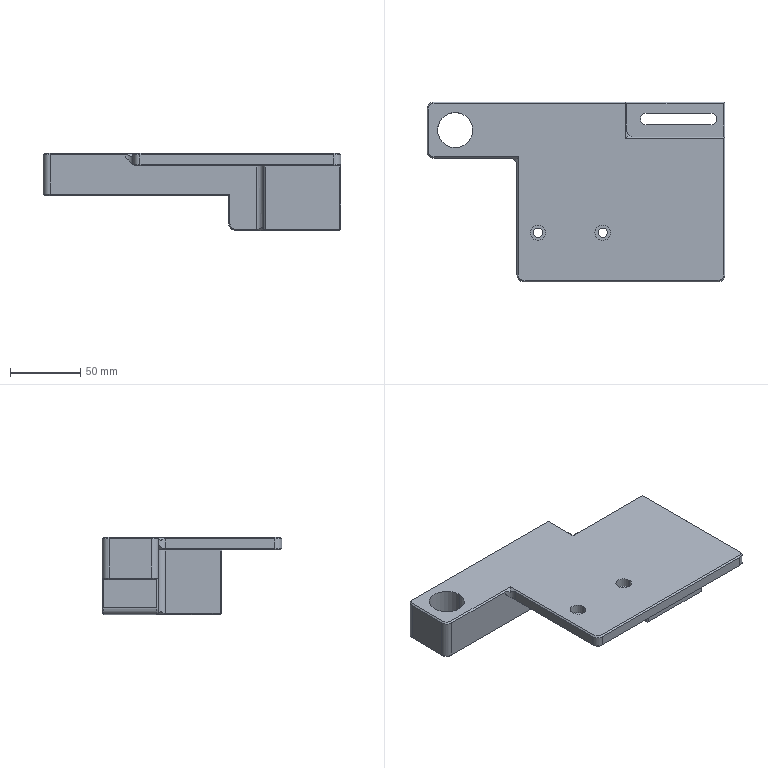NC program | NX | posted with a generic post | part box 212 x 128 x 55 mm
Lines 40 to 1041 of 7327:
(ZLEVEL_PROFILE , TOOL : D17R0.8)
N66 T19 M6
N68 G54
N70 G17 G0 G90 X-34.204 Y-75.847 S2000 M3
N72 G43 Z30. H19
N74 Z-0.299
N76 G94 G1 X-35.548 Y-73.385 F1000.
N78 G3 X-37. Y-72.5 R1.7
N80 G1 X-37.377 Y-72.491 F2000.
N82 X-39.204 Y-72.315
N84 G2 X-41.763 Y-71.628 R16.725
N86 X-44.137 Y-70.455 R17.555
N88 X-46.243 Y-68.833 R16.661
N90 X-48.008 Y-66.81 R16.904
N92 X-49.323 Y-64.502 R16.126
N94 X-50.15 Y-62.04 R17.33
N96 X-50.5 Y-59.144 R17.117
N98 G1 Y15.5
N100 X-100.985
N102 X-101.383 Y15.509
N104 X-103.25 Y15.692
N106 G2 X-105.769 Y16.375 R18.316
N108 X-110.251 Y19.173 R14.115
N110 X-111.999 Y21.178 R16.782
N112 X-113.297 Y23.438 R17.54
N114 X-114.152 Y25.971 R16.756
N116 X-114.49 Y28.605 R16.66
N118 G1 X-114.5 Y29.
N120 X-114.496 Y29.035
N122 X-114.498 Y30.056
N124 X-114.499 Y30.558
N126 G3 X-115.354 Y32.027 R1.7
N128 G1 X-117.608 Y33.32
N130 G0 X-117.607 Y33.322 Z-0.598
N132 G1 X-115.353 Y32.028 F1000.
N134 G2 X-114.499 Y30.558 R1.7
N136 G1 X-114.498 Y30.056 F2000.
N138 X-114.497 Y29.035
N140 X-114.5 Y29.
N142 X-114.49 Y28.605
N144 G3 X-114.152 Y25.971 R16.408
N146 X-113.297 Y23.438 R15.504
N148 X-111.999 Y21.178 R17.275
N150 X-110.251 Y19.173 R16.617
N152 X-105.769 Y16.375 R14.059
N154 X-103.25 Y15.692 R17.985
N156 G1 X-101.383 Y15.509
N158 X-100.985 Y15.5
N160 X-50.5
N162 Y-59.138
N164 G3 X-50.15 Y-62.04 R16.924
N166 G1 X-50.061 Y-62.353
N168 X-49.627 Y-63.765
N170 X-49.592 Y-63.858
N172 G3 X-48.318 Y-66.377 R16.221
N174 X-46.243 Y-68.833 R16.659
N176 X-44.137 Y-70.455 R16.48
N178 X-41.763 Y-71.628 R17.111
N180 X-39.204 Y-72.315 R16.672
N182 G1 X-37.377 Y-72.491
N184 X-37. Y-72.5
N186 G2 X-35.548 Y-73.385 R1.7
N188 G1 X-34.208 Y-75.839
N190 G0 X-34.207 Y-75.843 Z-0.897
N192 G1 X-35.548 Y-73.385 F1000.
N194 G3 X-37. Y-72.5 R1.7
N196 G1 X-37.377 Y-72.491 F2000.
N198 X-39.204 Y-72.315
N200 G2 X-41.763 Y-71.628 R16.772
N202 X-44.137 Y-70.455 R16.925
N204 X-46.243 Y-68.833 R16.304
N206 X-48.008 Y-66.81 R16.476
N208 X-50.134 Y-62.108 R13.885
N210 X-50.5 Y-59.121 R16.437
N212 G1 Y15.5
N214 X-100.985
N216 X-101.383 Y15.509
N218 X-103.25 Y15.692
N220 G2 X-105.769 Y16.375 R17.578
N222 X-110.251 Y19.173 R14.002
N224 X-111.999 Y21.178 R16.455
N226 X-113.297 Y23.438 R17.026
N228 X-114.152 Y25.971 R15.355
N230 X-114.49 Y28.605 R17.016
N232 G1 X-114.5 Y29.
N234 X-114.498 Y30.056
N236 X-114.499 Y30.558
N238 G3 X-115.352 Y32.028 R1.7
N240 G1 X-117.607 Y33.325
N242 G0 X-117.634 Y33.343 Z-1.196
N244 G1 X-115.351 Y32.029 F1000.
N246 G2 X-114.499 Y30.558 R1.7
N248 G1 Y30.056 F2000.
N250 X-114.5 Y29.
N252 X-114.49 Y28.605
N254 G3 X-114.152 Y25.971 R16.763
N256 X-112.816 Y22.397 R16.562
N258 X-110.251 Y19.173 R16.296
N260 X-105.769 Y16.375 R13.947
N262 X-103.218 Y15.687 R17.241
N264 G1 X-101.383 Y15.509
N266 X-100.985 Y15.5
N268 X-50.5
N270 Y-59.119
N272 G3 X-50.15 Y-62.04 R16.449
N274 X-49.323 Y-64.503 R16.842
N276 X-47.755 Y-67.18 R16.253
N278 X-44.137 Y-70.455 R14.338
N280 X-41.763 Y-71.628 R16.744
N282 X-39.204 Y-72.315 R16.566
N284 G1 X-37.377 Y-72.491
N286 X-37. Y-72.5
N288 G2 X-35.548 Y-73.385 R1.7
N290 G1 X-34.206 Y-75.844
N292 G0 X-34.205 Y-75.846 Z-1.495
N294 G1 X-35.548 Y-73.385 F1000.
N296 G3 X-37. Y-72.5 R1.7
N298 G1 X-37.377 Y-72.491 F2000.
N300 X-39.204 Y-72.315
N302 G2 X-41.763 Y-71.628 R16.392
N304 X-44.137 Y-70.455 R16.512
N306 X-47.853 Y-67.036 R14.045
N308 X-49.323 Y-64.503 R15.704
N310 X-50.15 Y-62.04 R16.586
N312 X-50.5 Y-59.105 R16.167
N314 G1 Y15.5
N316 X-100.985
N318 X-101.431 Y15.51
N320 X-103.25 Y15.692
N322 G2 X-105.769 Y16.375 R16.963
N324 X-110.251 Y19.173 R13.91
N326 X-112.823 Y22.412 R16.137
N328 X-114.152 Y25.971 R16.822
N330 X-114.49 Y28.605 R16.493
N332 G1 X-114.5 Y29.
N334 X-114.499 Y30.056
N336 Y30.558
N338 G3 X-115.35 Y32.029 R1.7
N340 G1 X-117.839 Y33.464
N342 G0 X-117.899 Y33.502 Z-1.793
N344 G1 X-115.349 Y32.03 F1000.
N346 G2 X-114.499 Y30.558 R1.7
N348 G1 Y30.056 F2000.
N350 X-114.5 Y29.
N352 G3 X-100.985 Y15.5 R13.507
N354 G1 X-50.5
N356 Y-59.882
N358 X-50.31 Y-61.241
N360 X-50.268 Y-61.476
N362 G3 X-37. Y-72.5 R13.504
N364 G2 X-35.528 Y-73.351 R1.7
N366 G1 X-34.058 Y-75.9
N368 G0 X-34.056 Z-2.092
N370 G1 X-35.528 Y-73.35 F1000.
N372 G3 X-37. Y-72.5 R1.7
N374 G2 X-50.5 Y-59. R13.5 F2000.
N376 G1 Y15.5
N378 X-101.
N380 G2 X-114.5 Y29. R13.5
N382 G1 Y29.553
N384 X-114.499 Y30.558
N386 G3 X-115.348 Y32.031 R1.7
N388 G1 X-117.9 Y33.507
N390 G0 Z-2.391
N392 G1 X-115.348 Y32.031 F1000.
N394 G2 X-114.499 Y30.558 R1.7
N396 G1 X-114.5 Y29.553 F2000.
N398 Y29.
N400 G3 X-101. Y15.5 R13.5
N402 G1 X-50.5
N404 Y-59.
N406 G3 X-37. Y-72.5 R13.5
N408 G2 X-35.528 Y-73.35 R1.7
N410 G1 X-34.056 Y-75.9
N412 G0 Z-2.69
N414 G1 X-35.528 Y-73.35 F1000.
N416 G3 X-37. Y-72.5 R1.7
N418 G2 X-50.5 Y-59. R13.5 F2000.
N420 G1 Y15.5
N422 X-101.
N424 G2 X-114.5 Y29. R13.5
N426 G1 Y29.553
N428 X-114.499 Y30.558
N430 G3 X-115.348 Y32.031 R1.7
N432 G1 X-117.9 Y33.507
N434 G0 Z-2.989
N436 G1 X-115.348 Y32.031 F1000.
N438 G2 X-114.499 Y30.558 R1.7
N440 G1 X-114.5 Y29.553 F2000.
N442 Y29.
N444 G3 X-101. Y15.5 R13.5
N446 G1 X-50.5
N448 Y-59.
N450 G3 X-37. Y-72.5 R13.5
N452 G2 X-35.528 Y-73.35 R1.7
N454 G1 X-34.056 Y-75.9
N456 G0 Z-3.288
N458 G1 X-35.528 Y-73.35 F1000.
N460 G3 X-37. Y-72.5 R1.7
N462 G2 X-50.5 Y-59. R13.5 F2000.
N464 G1 Y15.5
N466 X-101.
N468 G2 X-114.5 Y29. R13.5
N470 G1 Y29.553
N472 X-114.499 Y30.558
N474 G3 X-115.348 Y32.031 R1.7
N476 G1 X-117.9 Y33.507
N478 G0 Z-3.587
N480 G1 X-115.348 Y32.031 F1000.
N482 G2 X-114.499 Y30.558 R1.7
N484 G1 X-114.5 Y29.553 F2000.
N486 Y29.
N488 G3 X-101. Y15.5 R13.5
N490 G1 X-50.5
N492 Y-59.
N494 G3 X-37. Y-72.5 R13.5
N496 G2 X-35.528 Y-73.35 R1.7
N498 G1 X-34.056 Y-75.9
N500 G0 Z-3.886
N502 G1 X-35.528 Y-73.35 F1000.
N504 G3 X-37. Y-72.5 R1.7
N506 G2 X-50.5 Y-59. R13.5 F2000.
N508 G1 Y15.5
N510 X-101.
N512 G2 X-114.5 Y29. R13.5
N514 G1 Y29.553
N516 X-114.499 Y30.558
N518 G3 X-115.348 Y32.031 R1.7
N520 G1 X-117.9 Y33.507
N522 G0 Z-4.185
N524 G1 X-115.348 Y32.031 F1000.
N526 G2 X-114.499 Y30.558 R1.7
N528 G1 X-114.5 Y29.553 F2000.
N530 Y29.
N532 G3 X-101. Y15.5 R13.5
N534 G1 X-50.5
N536 Y-59.
N538 G3 X-37. Y-72.5 R13.5
N540 G2 X-35.528 Y-73.35 R1.7
N542 G1 X-34.056 Y-75.9
N544 G0 Z-4.484
N546 G1 X-35.528 Y-73.35 F1000.
N548 G3 X-37. Y-72.5 R1.7
N550 G2 X-50.5 Y-59. R13.5 F2000.
N552 G1 Y15.5
N554 X-101.
N556 G2 X-114.5 Y29. R13.5
N558 G1 Y29.553
N560 X-114.499 Y30.558
N562 G3 X-115.348 Y32.031 R1.7
N564 G1 X-117.9 Y33.507
N566 G0 Z-4.783
N568 G1 X-115.348 Y32.031 F1000.
N570 G2 X-114.499 Y30.558 R1.7
N572 G1 X-114.5 Y29.553 F2000.
N574 Y29.
N576 G3 X-101. Y15.5 R13.5
N578 G1 X-50.5
N580 Y-59.
N582 G3 X-37. Y-72.5 R13.5
N584 G2 X-35.528 Y-73.35 R1.7
N586 G1 X-34.056 Y-75.9
N588 G0 Z-5.082
N590 G1 X-35.528 Y-73.35 F1000.
N592 G3 X-37. Y-72.5 R1.7
N594 G2 X-50.5 Y-59. R13.5 F2000.
N596 G1 Y15.5
N598 X-101.
N600 G2 X-114.5 Y29. R13.5
N602 G1 Y29.553
N604 X-114.499 Y30.558
N606 G3 X-115.348 Y32.031 R1.7
N608 G1 X-117.9 Y33.507
N610 G0 Z-5.38
N612 G1 X-115.348 Y32.031 F1000.
N614 G2 X-114.499 Y30.558 R1.7
N616 G1 X-114.5 Y29.553 F2000.
N618 Y29.
N620 G3 X-101. Y15.5 R13.5
N622 G1 X-50.5
N624 Y-59.
N626 G3 X-37. Y-72.5 R13.5
N628 G2 X-35.528 Y-73.35 R1.7
N630 G1 X-34.056 Y-75.9
N632 G0 Z-5.679
N634 G1 X-35.528 Y-73.35 F1000.
N636 G3 X-37. Y-72.5 R1.7
N638 G2 X-50.5 Y-59. R13.5 F2000.
N640 G1 Y15.5
N642 X-101.
N644 G2 X-114.5 Y29. R13.5
N646 G1 Y29.553
N648 X-114.499 Y30.558
N650 G3 X-115.348 Y32.031 R1.7
N652 G1 X-117.9 Y33.507
N654 G0 Y33.506 Z-5.978
N656 G1 X-115.348 Y32.031 F1000.
N658 G2 X-114.499 Y30.558 R1.7
N660 G1 X-114.5 Y29.553 F2000.
N662 Y29.
N664 G3 X-101. Y15.5 R13.5
N666 G1 X-50.5
N668 Y-59.
N670 G3 X-37. Y-72.5 R13.5
N672 G2 X-35.528 Y-73.35 R1.7
N674 G1 X-34.056 Y-75.9
N676 G0 Z-6.277
N678 G1 X-35.528 Y-73.35 F1000.
N680 G3 X-37. Y-72.5 R1.7
N682 G2 X-50.5 Y-59. R13.5 F2000.
N684 G1 Y15.5
N686 X-101.
N688 G2 X-114.5 Y29. R13.5
N690 G1 Y29.553
N692 X-114.499 Y30.558
N694 G3 X-115.348 Y32.031 R1.7
N696 G1 X-117.9 Y33.506
N698 G0 Z-6.576
N700 G1 X-115.348 Y32.031 F1000.
N702 G2 X-114.499 Y30.558 R1.7
N704 G1 X-114.5 Y29.553 F2000.
N706 Y29.
N708 G3 X-101. Y15.5 R13.5
N710 G1 X-50.5
N712 Y-59.
N714 G3 X-37. Y-72.5 R13.5
N716 G2 X-35.528 Y-73.35 R1.7
N718 G1 X-34.056 Y-75.9
N720 G0 Z-6.875
N722 G1 X-35.528 Y-73.35 F1000.
N724 G3 X-37. Y-72.5 R1.7
N726 G2 X-50.5 Y-59. R13.5 F2000.
N728 G1 Y15.5
N730 X-101.
N732 G2 X-114.5 Y29. R13.5
N734 G1 Y29.553
N736 X-114.499 Y30.558
N738 G3 X-115.348 Y32.031 R1.7
N740 G1 X-117.9 Y33.506
N742 G0 Z-7.174
N744 G1 X-115.348 Y32.031 F1000.
N746 G2 X-114.499 Y30.558 R1.7
N748 G1 X-114.5 Y29.553 F2000.
N750 Y29.
N752 G3 X-101. Y15.5 R13.5
N754 G1 X-50.5
N756 Y-59.
N758 G3 X-37. Y-72.5 R13.5
N760 G2 X-35.528 Y-73.35 R1.7
N762 G1 X-34.056 Y-75.9
N764 G0 Z-7.473
N766 G1 X-35.528 Y-73.35 F1000.
N768 G3 X-37. Y-72.5 R1.7
N770 G2 X-50.5 Y-59. R13.5 F2000.
N772 G1 Y15.5
N774 X-101.
N776 G2 X-114.5 Y29. R13.5
N778 G1 Y29.553
N780 X-114.499 Y30.558
N782 G3 X-115.348 Y32.031 R1.7
N784 G1 X-117.9 Y33.506
N786 G0 Z-7.772
N788 G1 X-115.348 Y32.031 F1000.
N790 G2 X-114.499 Y30.558 R1.7
N792 G1 X-114.5 Y29.553 F2000.
N794 Y29.
N796 G3 X-101. Y15.5 R13.5
N798 G1 X-50.5
N800 Y-59.
N802 G3 X-37. Y-72.5 R13.5
N804 G2 X-35.528 Y-73.35 R1.7
N806 G1 X-34.056 Y-75.9
N808 G0 Z-8.071
N810 G1 X-35.528 Y-73.35 F1000.
N812 G3 X-37. Y-72.5 R1.7
N814 G2 X-50.5 Y-59. R13.5 F2000.
N816 G1 Y15.5
N818 X-101.
N820 G2 X-114.5 Y29. R13.5
N822 G1 Y29.553
N824 X-114.499 Y30.558
N826 G3 X-115.348 Y32.031 R1.7
N828 G1 X-117.9 Y33.506
N830 G0 Z-8.37
N832 G1 X-115.348 Y32.031 F1000.
N834 G2 X-114.499 Y30.558 R1.7
N836 G1 X-114.5 Y29.553 F2000.
N838 Y29.
N840 G3 X-101. Y15.5 R13.5
N842 G1 X-50.5
N844 Y-59.
N846 G3 X-37. Y-72.5 R13.5
N848 G2 X-35.528 Y-73.35 R1.7
N850 G1 X-34.056 Y-75.9
N852 G0 Z-8.668
N854 G1 X-35.528 Y-73.35 F1000.
N856 G3 X-37. Y-72.5 R1.7
N858 G2 X-50.5 Y-59. R13.5 F2000.
N860 G1 Y15.5
N862 X-101.
N864 G2 X-114.5 Y29. R13.5
N866 G1 Y29.553
N868 X-114.499 Y30.558
N870 G3 X-115.348 Y32.031 R1.7
N872 G1 X-117.9 Y33.506
N874 G0 Z-8.967
N876 G1 X-115.348 Y32.031 F1000.
N878 G2 X-114.499 Y30.558 R1.7
N880 G1 X-114.5 Y29.553 F2000.
N882 Y29.
N884 G3 X-101. Y15.5 R13.5
N886 G1 X-50.5
N888 Y-59.
N890 G3 X-37. Y-72.5 R13.5
N892 G2 X-35.528 Y-73.35 R1.7
N894 G1 X-34.056 Y-75.9
N896 G0 Z-9.266
N898 G1 X-35.528 Y-73.35 F1000.
N900 G3 X-37. Y-72.5 R1.7
N902 G2 X-50.5 Y-59. R13.5 F2000.
N904 G1 Y15.5
N906 X-101.
N908 G2 X-114.5 Y29. R13.5
N910 G1 Y29.553
N912 X-114.499 Y30.558
N914 G3 X-115.348 Y32.031 R1.7
N916 G1 X-117.9 Y33.506
N918 G0 Z-9.565
N920 G1 X-115.348 Y32.031 F1000.
N922 G2 X-114.499 Y30.558 R1.7
N924 G1 X-114.5 Y29.553 F2000.
N926 Y29.
N928 G3 X-101. Y15.5 R13.5
N930 G1 X-50.5
N932 Y-59.
N934 G3 X-37. Y-72.5 R13.5
N936 G2 X-35.528 Y-73.35 R1.7
N938 G1 X-34.056 Y-75.9
N940 G0 Z-9.864
N942 G1 X-35.528 Y-73.35 F1000.
N944 G3 X-37. Y-72.5 R1.7
N946 G2 X-50.5 Y-59. R13.5 F2000.
N948 G1 Y15.5
N950 X-101.
N952 G2 X-114.5 Y29. R13.5
N954 G1 Y29.553
N956 X-114.499 Y30.558
N958 G3 X-115.348 Y32.031 R1.7
N960 G1 X-117.9 Y33.506
N962 G0 Z-10.163
N964 G1 X-115.348 Y32.031 F1000.
N966 G2 X-114.499 Y30.558 R1.7
N968 G1 X-114.5 Y29.553 F2000.
N970 Y29.
N972 G3 X-101. Y15.5 R13.5
N974 G1 X-50.5
N976 Y-59.
N978 G3 X-37. Y-72.5 R13.5
N980 G2 X-35.528 Y-73.35 R1.7
N982 G1 X-34.056 Y-75.9
N984 G0 Z-10.462
N986 G1 X-35.528 Y-73.35 F1000.
N988 G3 X-37. Y-72.5 R1.7
N990 G2 X-50.5 Y-59. R13.5 F2000.
N992 G1 Y15.5
N994 X-101.
N996 G2 X-114.5 Y29. R13.5
N998 G1 Y29.553
N1000 X-114.499 Y30.558
N1002 G3 X-115.348 Y32.031 R1.7
N1004 G1 X-117.9 Y33.506
N1006 G0 Z-10.761
N1008 G1 X-115.348 Y32.031 F1000.
N1010 G2 X-114.499 Y30.558 R1.7
N1012 G1 X-114.5 Y29.553 F2000.
N1014 Y29.
N1016 G3 X-101. Y15.5 R13.5
N1018 G1 X-50.5
N1020 Y-59.
N1022 G3 X-37. Y-72.5 R13.5
N1024 G2 X-35.528 Y-73.35 R1.7
N1026 G1 X-34.056 Y-75.9
N1028 G0 Z-11.06
N1030 G1 X-35.528 Y-73.35 F1000.
N1032 G3 X-37. Y-72.5 R1.7
N1034 G2 X-50.5 Y-59. R13.5 F2000.
N1036 G1 Y15.5
N1038 X-101.
N1040 G2 X-114.5 Y29. R13.5
N1042 G1 Y29.553
N1044 X-114.499 Y30.558
N1046 G3 X-115.348 Y32.031 R1.7
N1048 G1 X-117.9 Y33.506
N1050 G0 Z-11.359
N1052 G1 X-115.348 Y32.03 F1000.
N1054 G2 X-114.499 Y30.558 R1.7
N1056 G1 X-114.5 Y29.553 F2000.
N1058 Y29.
N1060 G3 X-101. Y15.5 R13.5
N1062 G1 X-50.5
N1064 Y-59.
N1066 G3 X-37. Y-72.5 R13.5
N1068 G2 X-35.528 Y-73.35 R1.7
N1070 G1 X-34.056 Y-75.9
N1072 G0 Z-11.658
N1074 G1 X-35.528 Y-73.35 F1000.
N1076 G3 X-37. Y-72.5 R1.7
N1078 G2 X-50.5 Y-59. R13.5 F2000.
N1080 G1 Y15.5
N1082 X-101.
N1084 G2 X-114.5 Y29. R13.5
N1086 G1 Y29.553
N1088 X-114.499 Y30.558
N1090 G3 X-115.348 Y32.03 R1.7
N1092 G1 X-117.9 Y33.506
N1094 G0 Z-11.957
N1096 G1 X-115.348 Y32.03 F1000.
N1098 G2 X-114.499 Y30.558 R1.7
N1100 G1 X-114.5 Y29.553 F2000.
N1102 Y29.
N1104 G3 X-101. Y15.5 R13.5
N1106 G1 X-50.5
N1108 Y-59.
N1110 G3 X-37. Y-72.5 R13.5
N1112 G2 X-35.528 Y-73.35 R1.7
N1114 G1 X-34.056 Y-75.9
N1116 G0 Z-12.255
N1118 G1 X-35.528 Y-73.35 F1000.
N1120 G3 X-37. Y-72.5 R1.7
N1122 G2 X-50.5 Y-59. R13.5 F2000.
N1124 G1 Y15.5
N1126 X-101.
N1128 G2 X-114.5 Y29. R13.5
N1130 G1 Y29.553
N1132 X-114.499 Y30.558
N1134 G3 X-115.349 Y32.03 R1.7
N1136 G1 X-117.9 Y33.506
N1138 G0 Z-12.554
N1140 G1 X-115.349 Y32.03 F1000.
N1142 G2 X-114.499 Y30.558 R1.7
N1144 G1 X-114.5 Y29.553 F2000.
N1146 Y29.
N1148 G3 X-101. Y15.5 R13.5
N1150 G1 X-50.5
N1152 Y-59.
N1154 G3 X-37. Y-72.5 R13.5
N1156 G2 X-35.528 Y-73.35 R1.7
N1158 G1 X-34.056 Y-75.9
N1160 G0 Z-12.853
N1162 G1 X-35.528 Y-73.35 F1000.
N1164 G3 X-37. Y-72.5 R1.7
N1166 G2 X-50.5 Y-59. R13.5 F2000.
N1168 G1 Y15.5
N1170 X-101.
N1172 G2 X-114.5 Y29. R13.5
N1174 G1 Y29.553
N1176 X-114.499 Y30.558
N1178 G3 X-115.349 Y32.03 R1.7
N1180 G1 X-117.9 Y33.506
N1182 G0 Z-13.152
N1184 G1 X-115.349 Y32.03 F1000.
N1186 G2 X-114.499 Y30.558 R1.7
N1188 G1 X-114.5 Y29.553 F2000.
N1190 Y29.
N1192 G3 X-101. Y15.5 R13.5
N1194 G1 X-50.5
N1196 Y-59.
N1198 G3 X-37. Y-72.5 R13.5
N1200 G2 X-35.528 Y-73.35 R1.7
N1202 G1 X-34.056 Y-75.9
N1204 G0 Z-13.451
N1206 G1 X-35.528 Y-73.35 F1000.
N1208 G3 X-37. Y-72.5 R1.7
N1210 G2 X-50.5 Y-59. R13.5 F2000.
N1212 G1 Y15.5
N1214 X-101.
N1216 G2 X-114.5 Y29. R13.5
N1218 G1 Y29.553
N1220 X-114.499 Y30.558
N1222 G3 X-115.349 Y32.03 R1.7
N1224 G1 X-117.9 Y33.505
N1226 G0 Z-13.75
N1228 G1 X-115.349 Y32.03 F1000.
N1230 G2 X-114.499 Y30.558 R1.7
N1232 G1 X-114.5 Y29.553 F2000.
N1234 Y29.
N1236 G3 X-101. Y15.5 R13.5
N1238 G1 X-50.5
N1240 Y-59.
N1242 G3 X-37. Y-72.5 R13.5
N1244 G2 X-35.528 Y-73.35 R1.7
N1246 G1 X-34.056 Y-75.9
N1248 G0 Z-14.049
N1250 G1 X-35.528 Y-73.35 F1000.
N1252 G3 X-37. Y-72.5 R1.7
N1254 G2 X-50.5 Y-59. R13.5 F2000.
N1256 G1 Y15.5
N1258 X-101.
N1260 G2 X-114.5 Y29. R13.5
N1262 G1 Y29.553
N1264 X-114.499 Y30.558
N1266 G3 X-115.349 Y32.03 R1.7
N1268 G1 X-117.9 Y33.505
N1270 G0 Z-14.348
N1272 G1 X-115.349 Y32.03 F1000.
N1274 G2 X-114.499 Y30.558 R1.7
N1276 G1 X-114.5 Y29.553 F2000.
N1278 Y29.
N1280 G3 X-101. Y15.5 R13.5
N1282 G1 X-50.5
N1284 Y-59.
N1286 G3 X-37. Y-72.5 R13.5
N1288 G2 X-35.528 Y-73.35 R1.7
N1290 G1 X-34.056 Y-75.9
N1292 G0 Z-14.647
N1294 G1 X-35.528 Y-73.35 F1000.
N1296 G3 X-37. Y-72.5 R1.7
N1298 G2 X-50.5 Y-59. R13.5 F2000.
N1300 G1 Y15.5
N1302 X-101.
N1304 G2 X-114.5 Y29. R13.5
N1306 G1 Y29.553
N1308 X-114.499 Y30.558
N1310 G3 X-115.349 Y32.03 R1.7
N1312 G1 X-117.9 Y33.505
N1314 G0 Z-14.946
N1316 G1 X-115.349 Y32.03 F1000.
N1318 G2 X-114.499 Y30.558 R1.7
N1320 G1 X-114.5 Y29.553 F2000.
N1322 Y29.
N1324 G3 X-101. Y15.5 R13.5
N1326 G1 X-50.5
N1328 Y-59.
N1330 G3 X-37. Y-72.5 R13.5
N1332 G2 X-35.528 Y-73.35 R1.7
N1334 G1 X-34.056 Y-75.9
N1336 G0 Z-15.245
N1338 G1 X-35.528 Y-73.35 F1000.
N1340 G3 X-37. Y-72.5 R1.7
N1342 G2 X-50.5 Y-59. R13.5 F2000.
N1344 G1 Y15.5
N1346 X-101.
N1348 G2 X-114.5 Y29. R13.5
N1350 G1 Y29.553
N1352 X-114.499 Y30.558
N1354 G3 X-115.349 Y32.03 R1.7
N1356 G1 X-117.9 Y33.505
N1358 G0 Z-15.543
N1360 G1 X-115.349 Y32.03 F1000.
N1362 G2 X-114.499 Y30.558 R1.7
N1364 G1 X-114.5 Y29.553 F2000.
N1366 Y29.
N1368 G3 X-101. Y15.5 R13.5
N1370 G1 X-50.5
N1372 Y-59.
N1374 G3 X-37. Y-72.5 R13.5
N1376 G2 X-35.528 Y-73.35 R1.7
N1378 G1 X-34.056 Y-75.9
N1380 G0 Z-15.842
N1382 G1 X-35.528 Y-73.35 F1000.
N1384 G3 X-37. Y-72.5 R1.7
N1386 G2 X-50.5 Y-59. R13.5 F2000.
N1388 G1 Y15.5
N1390 X-101.
N1392 G2 X-114.5 Y29. R13.5
N1394 G1 Y29.553
N1396 X-114.499 Y30.558
N1398 G3 X-115.349 Y32.03 R1.7
N1400 G1 X-117.9 Y33.505
N1402 G0 Z-16.141
N1404 G1 X-115.349 Y32.03 F1000.
N1406 G2 X-114.499 Y30.558 R1.7
N1408 G1 X-114.5 Y29.553 F2000.
N1410 Y29.
N1412 G3 X-101. Y15.5 R13.5
N1414 G1 X-50.5
N1416 Y-59.
N1418 G3 X-37. Y-72.5 R13.5
N1420 G2 X-35.528 Y-73.35 R1.7
N1422 G1 X-34.056 Y-75.9
N1424 G0 Z-16.44
N1426 G1 X-35.528 Y-73.35 F1000.
N1428 G3 X-37. Y-72.5 R1.7
N1430 G2 X-50.5 Y-59. R13.5 F2000.
N1432 G1 Y15.5
N1434 X-101.
N1436 G2 X-114.5 Y29. R13.5
N1438 G1 Y29.553
N1440 X-114.499 Y30.558
N1442 G3 X-115.349 Y32.03 R1.7
N1444 G1 X-117.9 Y33.505
N1446 G0 Z-16.739
N1448 G1 X-115.349 Y32.03 F1000.
N1450 G2 X-114.5 Y30.558 R1.7
N1452 G1 Y29.553 F2000.
N1454 Y29.
N1456 G3 X-101. Y15.5 R13.5
N1458 G1 X-50.5
N1460 Y-59.
N1462 G3 X-37. Y-72.5 R13.5
N1464 G2 X-35.528 Y-73.35 R1.7
N1466 G1 X-34.056 Y-75.9
N1468 G0 Z-17.038
N1470 G1 X-35.528 Y-73.35 F1000.
N1472 G3 X-37. Y-72.5 R1.7
N1474 G2 X-50.5 Y-59. R13.5 F2000.
N1476 G1 Y15.5
N1478 X-101.
N1480 G2 X-114.5 Y29. R13.5
N1482 G1 Y29.553
N1484 Y30.558
N1486 G3 X-115.349 Y32.03 R1.7
N1488 G1 X-117.9 Y33.505
N1490 G0 Z-17.337
N1492 G1 X-115.349 Y32.03 F1000.
N1494 G2 X-114.5 Y30.558 R1.7
N1496 G1 Y29.553 F2000.
N1498 Y29.
N1500 G3 X-101. Y15.5 R13.5
N1502 G1 X-50.5
N1504 Y-59.
N1506 G3 X-37. Y-72.5 R13.5
N1508 G2 X-35.528 Y-73.35 R1.7
N1510 G1 X-34.056 Y-75.9
N1512 G0 Z-17.636
N1514 G1 X-35.528 Y-73.35 F1000.
N1516 G3 X-37. Y-72.5 R1.7
N1518 G2 X-50.5 Y-59. R13.5 F2000.
N1520 G1 Y15.5
N1522 X-101.
N1524 G2 X-114.5 Y29. R13.5
N1526 G1 Y29.553
N1528 Y30.558
N1530 G3 X-115.349 Y32.03 R1.7
N1532 G1 X-117.9 Y33.505
N1534 G0 Z-17.935
N1536 G1 X-115.349 Y32.03 F1000.
N1538 G2 X-114.5 Y30.558 R1.7
N1540 G1 Y29.553 F2000.
N1542 Y29.
N1544 G3 X-101. Y15.5 R13.5
N1546 G1 X-50.5
N1548 Y-59.
N1550 G3 X-37. Y-72.5 R13.5
N1552 G2 X-35.528 Y-73.35 R1.7
N1554 G1 X-34.056 Y-75.9
N1556 G0 Z-18.234
N1558 G1 X-35.528 Y-73.35 F1000.
N1560 G3 X-37. Y-72.5 R1.7
N1562 G2 X-50.5 Y-59. R13.5 F2000.
N1564 G1 Y15.5
N1566 X-101.
N1568 G2 X-114.5 Y29. R13.5
N1570 G1 Y29.553
N1572 Y30.558
N1574 G3 X-115.349 Y32.03 R1.7
N1576 G1 X-117.9 Y33.505
N1578 G0 Z-18.533
N1580 G1 X-115.349 Y32.03 F1000.
N1582 G2 X-114.5 Y30.558 R1.7
N1584 G1 Y29.553 F2000.
N1586 Y29.
N1588 G3 X-101. Y15.5 R13.5
N1590 G1 X-50.5
N1592 Y-59.
N1594 G3 X-37. Y-72.5 R13.5
N1596 G2 X-35.528 Y-73.35 R1.7
N1598 G1 X-34.056 Y-75.9
N1600 G0 Z-18.832
N1602 G1 X-35.528 Y-73.35 F1000.
N1604 G3 X-37. Y-72.5 R1.7
N1606 G2 X-50.5 Y-59. R13.5 F2000.
N1608 G1 Y15.5
N1610 X-101.
N1612 G2 X-114.5 Y29. R13.5
N1614 G1 Y29.553
N1616 Y30.558
N1618 G3 X-115.349 Y32.03 R1.7
N1620 G1 X-117.9 Y33.505
N1622 G0 Z-19.13
N1624 G1 X-115.349 Y32.03 F1000.
N1626 G2 X-114.5 Y30.558 R1.7
N1628 G1 Y29.553 F2000.
N1630 Y29.
N1632 G3 X-101. Y15.5 R13.5
N1634 G1 X-50.5
N1636 Y-59.
N1638 G3 X-37. Y-72.5 R13.5
N1640 G2 X-35.528 Y-73.35 R1.7
N1642 G1 X-34.056 Y-75.9
N1644 G0 Z-19.429
N1646 G1 X-35.528 Y-73.35 F1000.
N1648 G3 X-37. Y-72.5 R1.7
N1650 G2 X-50.5 Y-59. R13.5 F2000.
N1652 G1 Y15.5
N1654 X-101.
N1656 G2 X-114.5 Y29. R13.5
N1658 G1 Y29.553
N1660 Y30.558
N1662 G3 X-115.349 Y32.03 R1.7
N1664 G1 X-117.9 Y33.505
N1666 G0 Z-19.728
N1668 G1 X-115.349 Y32.03 F1000.
N1670 G2 X-114.5 Y30.558 R1.7
N1672 G1 Y29.553 F2000.
N1674 Y29.
N1676 G3 X-101. Y15.5 R13.5
N1678 G1 X-50.5
N1680 Y-59.
N1682 G3 X-37. Y-72.5 R13.5
N1684 G2 X-35.528 Y-73.35 R1.7
N1686 G1 X-34.056 Y-75.9
N1688 G0 Z-20.027
N1690 G1 X-35.528 Y-73.35 F1000.
N1692 G3 X-37. Y-72.5 R1.7
N1694 G2 X-50.5 Y-59. R13.5 F2000.
N1696 G1 Y15.5
N1698 X-101.
N1700 G2 X-114.5 Y29. R13.5
N1702 G1 Y29.553
N1704 Y30.558
N1706 G3 X-115.349 Y32.03 R1.7
N1708 G1 X-117.9 Y33.505
N1710 G0 Z-20.326
N1712 G1 X-115.349 Y32.03 F1000.
N1714 G2 X-114.5 Y30.558 R1.7
N1716 G1 Y29.553 F2000.
N1718 Y29.
N1720 G3 X-101. Y15.5 R13.5
N1722 G1 X-50.5
N1724 Y-59.
N1726 G3 X-37. Y-72.5 R13.5
N1728 G2 X-35.528 Y-73.35 R1.7
N1730 G1 X-34.056 Y-75.9
N1732 G0 Z-20.625
N1734 G1 X-35.528 Y-73.35 F1000.
N1736 G3 X-37. Y-72.5 R1.7
N1738 G2 X-50.5 Y-59. R13.5 F2000.
N1740 G1 Y15.5
N1742 X-101.
N1744 G2 X-114.5 Y29. R13.5
N1746 G1 Y29.553
N1748 Y30.558
N1750 G3 X-115.349 Y32.03 R1.7
N1752 G1 X-117.9 Y33.505
N1754 G0 Y33.504 Z-20.924
N1756 G1 X-115.349 Y32.03 F1000.
N1758 G2 X-114.5 Y30.558 R1.7
N1760 G1 Y29.553 F2000.
N1762 Y29.
N1764 G3 X-101. Y15.5 R13.5
N1766 G1 X-50.5
N1768 Y-59.
N1770 G3 X-37. Y-72.5 R13.5
N1772 G2 X-35.528 Y-73.35 R1.7
N1774 G1 X-34.056 Y-75.9
N1776 G0 Z-21.223
N1778 G1 X-35.528 Y-73.35 F1000.
N1780 G3 X-37. Y-72.5 R1.7
N1782 G2 X-50.5 Y-59. R13.5 F2000.
N1784 G1 Y15.5
N1786 X-101.
N1788 G2 X-114.5 Y29. R13.5
N1790 G1 Y29.553
N1792 Y30.558
N1794 G3 X-115.349 Y32.03 R1.7
N1796 G1 X-117.9 Y33.504
N1798 G0 Z-21.522
N1800 G1 X-115.349 Y32.03 F1000.
N1802 G2 X-114.5 Y30.558 R1.7
N1804 G1 Y29.553 F2000.
N1806 Y29.
N1808 G3 X-101. Y15.5 R13.5
N1810 G1 X-50.5
N1812 Y-59.
N1814 G3 X-37. Y-72.5 R13.5
N1816 G2 X-35.528 Y-73.35 R1.7
N1818 G1 X-34.056 Y-75.9
N1820 G0 Z-21.821
N1822 G1 X-35.528 Y-73.35 F1000.
N1824 G3 X-37. Y-72.5 R1.7
N1826 G2 X-50.5 Y-59. R13.5 F2000.
N1828 G1 Y15.5
N1830 X-101.
N1832 G2 X-114.5 Y29. R13.5
N1834 G1 Y29.553
N1836 Y30.558
N1838 G3 X-115.349 Y32.03 R1.7
N1840 G1 X-117.9 Y33.504
N1842 G0 Z-22.12
N1844 G1 X-115.349 Y32.03 F1000.
N1846 G2 X-114.5 Y30.558 R1.7
N1848 G1 Y29.553 F2000.
N1850 Y29.
N1852 G3 X-101. Y15.5 R13.5
N1854 G1 X-50.5
N1856 Y-59.
N1858 G3 X-37. Y-72.5 R13.5
N1860 G2 X-35.528 Y-73.35 R1.7
N1862 G1 X-34.056 Y-75.9
N1864 G0 Z-22.418
N1866 G1 X-35.528 Y-73.35 F1000.
N1868 G3 X-37. Y-72.5 R1.7
N1870 G2 X-50.5 Y-59. R13.5 F2000.
N1872 G1 Y15.5
N1874 X-101.
N1876 G2 X-114.5 Y29. R13.5
N1878 G1 Y29.553
N1880 Y30.558
N1882 G3 X-115.349 Y32.03 R1.7
N1884 G1 X-117.9 Y33.504
N1886 G0 Z-22.717
N1888 G1 X-115.349 Y32.03 F1000.
N1890 G2 X-114.5 Y30.558 R1.7
N1892 G1 Y29.553 F2000.
N1894 Y29.
N1896 G3 X-101. Y15.5 R13.5
N1898 G1 X-50.5
N1900 Y-59.
N1902 G3 X-37. Y-72.5 R13.5
N1904 G2 X-35.528 Y-73.35 R1.7
N1906 G1 X-34.056 Y-75.9
N1908 G0 Z-23.016
N1910 G1 X-35.528 Y-73.35 F1000.
N1912 G3 X-37. Y-72.5 R1.7
N1914 G2 X-50.5 Y-59. R13.5 F2000.
N1916 G1 Y15.5
N1918 X-101.
N1920 G2 X-114.5 Y29. R13.5
N1922 G1 Y29.553
N1924 Y30.558
N1926 G3 X-115.349 Y32.03 R1.7
N1928 G1 X-117.9 Y33.504
N1930 G0 Z-23.315
N1932 G1 X-115.349 Y32.03 F1000.
N1934 G2 X-114.5 Y30.558 R1.7
N1936 G1 Y29.553 F2000.
N1938 Y29.
N1940 G3 X-101. Y15.5 R13.5
N1942 G1 X-50.5
N1944 Y-59.
N1946 G3 X-37. Y-72.5 R13.5
N1948 G2 X-35.528 Y-73.35 R1.7
N1950 G1 X-34.056 Y-75.9
N1952 G0 Z-23.614
N1954 G1 X-35.528 Y-73.35 F1000.
N1956 G3 X-37. Y-72.5 R1.7
N1958 G2 X-50.5 Y-59. R13.5 F2000.
N1960 G1 Y15.5
N1962 X-101.
N1964 G2 X-114.5 Y29. R13.5
N1966 G1 Y29.553
N1968 Y30.558
N1970 G3 X-115.349 Y32.03 R1.7
N1972 G1 X-117.9 Y33.504
N1974 G0 Z-23.913
N1976 G1 X-115.349 Y32.03 F1000.
N1978 G2 X-114.5 Y30.558 R1.7
N1980 G1 Y29.553 F2000.
N1982 Y29.
N1984 G3 X-101. Y15.5 R13.5
N1986 G1 X-50.5
N1988 Y-59.
N1990 G3 X-37. Y-72.5 R13.5
N1992 G2 X-35.528 Y-73.35 R1.7
N1994 G1 X-34.056 Y-75.9
N1996 G0 Z-24.212
N1998 G1 X-35.528 Y-73.35 F1000.
N2000 G3 X-37. Y-72.5 R1.7
N2002 G2 X-50.5 Y-59. R13.5 F2000.
N2004 G1 Y15.5
N2006 X-101.
N2008 G2 X-114.5 Y29. R13.5
N2010 G1 Y29.553
N2012 Y30.558
N2014 G3 X-115.349 Y32.03 R1.7
N2016 G1 X-117.9 Y33.504
N2018 G0 Z-24.511
N2020 G1 X-115.349 Y32.03 F1000.
N2022 G2 X-114.5 Y30.558 R1.7
N2024 G1 Y29.553 F2000.
N2026 Y29.
N2028 G3 X-101. Y15.5 R13.5
N2030 G1 X-50.5
N2032 Y-59.
N2034 G3 X-37. Y-72.5 R13.5
N2036 G2 X-35.528 Y-73.35 R1.7
N2038 G1 X-34.056 Y-75.9
N2040 G0 Z-24.81
N2042 G1 X-35.528 Y-73.35 F1000.
N2044 G3 X-37. Y-72.5 R1.7
N2046 G2 X-50.5 Y-59. R13.5 F2000.
N2048 G1 Y15.5
N2050 X-101.
N2052 G2 X-114.5 Y29. R13.5
N2054 G1 Y29.553
N2056 Y30.558
N2058 G3 X-115.349 Y32.03 R1.7
N2060 G1 X-117.9 Y33.504
N2062 G0 Z-25.109